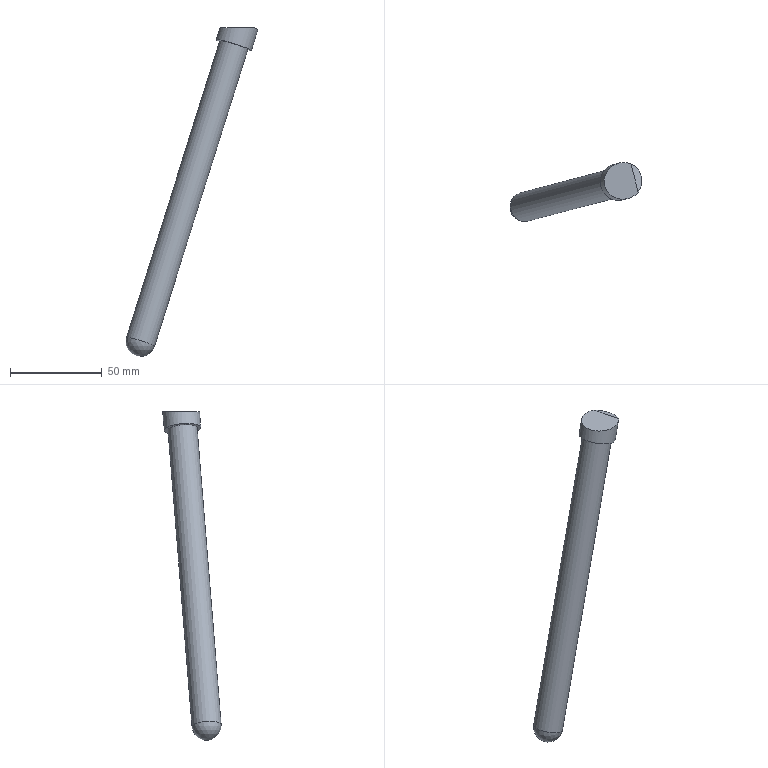Part | STEP file | 车灯-后视镜_id10_x_t | 1 solid | 6 faces | box 72 x 31.93 x 179.239 mm | volume 38387 mm3 | plane 3 | cylinder 2 | sphere 1 | commonest cylinder face diameters 16 x1 20 x1
STEP:
#1=CARTESIAN_POINT('',(-131.667,-129.696,-20.839));
#2=VERTEX_POINT('',#1);
#3=CARTESIAN_POINT('',(-124.036,-129.696,-23.239));
#4=DIRECTION('',(0.2992,0.07718,0.9511));
#5=DIRECTION('',(-0.9539,0.,0.3001));
#6=AXIS2_PLACEMENT_3D('',#3,#4,#5);
#7=CIRCLE('',#6,8.);
#8=EDGE_CURVE('',#2,#2,#7,.T.);
#9=ORIENTED_EDGE('',*,*,#8,.T.);
#10=EDGE_LOOP('',(#9));
#11=FACE_BOUND('',#10,.T.);
#12=CARTESIAN_POINT('',(-65.537,-116.575,136.039));
#13=VERTEX_POINT('',#12);
#14=CARTESIAN_POINT('',(-73.168,-116.575,138.44));
#15=DIRECTION('',(-0.2992,-0.07718,-0.9511));
#16=DIRECTION('',(0.9539,0.,-0.3001));
#17=AXIS2_PLACEMENT_3D('',#14,#15,#16);
#18=CIRCLE('',#17,8.);
#19=EDGE_CURVE('',#13,#13,#18,.T.);
#20=ORIENTED_EDGE('',*,*,#19,.T.);
#21=EDGE_LOOP('',(#20));
#22=FACE_BOUND('',#21,.T.);
#23=CARTESIAN_POINT('',(-92.019,-121.437,78.524));
#24=DIRECTION('',(-0.2992,-0.07718,-0.9511));
#25=DIRECTION('',(-0.9541,0.01184,0.2992));
#26=AXIS2_PLACEMENT_3D('',#23,#24,#25);
#27=CYLINDRICAL_SURFACE('',#26,8.);
#28=ADVANCED_FACE('',(#11,#22),#27,.T.);
#29=ORIENTED_EDGE('',*,*,#8,.F.);
#30=EDGE_LOOP('',(#29));
#31=FACE_OUTER_BOUND('',#30,.T.);
#32=CARTESIAN_POINT('',(-124.036,-129.696,-23.239));
#33=DIRECTION('',(0.,0.,1.));
#34=DIRECTION('',(1.,0.,0.));
#35=AXIS2_PLACEMENT_3D('',#32,#33,#34);
#36=SPHERICAL_SURFACE('',#35,8.);
#37=ADVANCED_FACE('',(#31),#36,.T.);
#38=CARTESIAN_POINT('',(-82.707,-116.575,141.441));
#39=VERTEX_POINT('',#38);
#40=CARTESIAN_POINT('',(-73.168,-116.575,138.44));
#41=DIRECTION('',(-0.2992,-0.07718,-0.9511));
#42=DIRECTION('',(-0.9539,0.,0.3001));
#43=AXIS2_PLACEMENT_3D('',#40,#41,#42);
#44=CIRCLE('',#43,10.);
#45=EDGE_CURVE('',#39,#39,#44,.T.);
#46=ORIENTED_EDGE('',*,*,#45,.T.);
#47=EDGE_LOOP('',(#46));
#48=FACE_BOUND('',#47,.T.);
#49=ORIENTED_EDGE('',*,*,#19,.F.);
#50=EDGE_LOOP('',(#49));
#51=FACE_BOUND('',#50,.T.);
#52=CARTESIAN_POINT('',(-73.168,-116.575,138.44));
#53=DIRECTION('',(0.2992,0.07718,0.9511));
#54=DIRECTION('',(0.9539,0.,-0.3001));
#55=AXIS2_PLACEMENT_3D('',#52,#53,#54);
#56=PLANE('',#55);
#57=ADVANCED_FACE('',(#48,#51),#56,.F.);
#58=CARTESIAN_POINT('',(-66.054,-106.475,148.));
#59=VERTEX_POINT('',#58);
#60=CARTESIAN_POINT('',(-62.057,-121.974,148.));
#61=VERTEX_POINT('',#60);
#62=CARTESIAN_POINT('',(-70.16,-115.799,148.));
#63=DIRECTION('',(0.,0.,1.));
#64=DIRECTION('',(-0.9683,-0.2498,0.));
#65=AXIS2_PLACEMENT_3D('',#62,#63,#64);
#66=ELLIPSE('',#65,10.515,10.);
#67=EDGE_CURVE('',#59,#61,#66,.T.);
#68=ORIENTED_EDGE('',*,*,#67,.F.);
#69=CARTESIAN_POINT('',(-69.577,-115.649,149.853));
#70=DIRECTION('',(-0.2992,-0.07718,-0.9511));
#71=DIRECTION('',(-0.9539,0.,0.3001));
#72=AXIS2_PLACEMENT_3D('',#69,#70,#71);
#73=CIRCLE('',#72,10.);
#74=EDGE_CURVE('',#59,#61,#73,.T.);
#75=ORIENTED_EDGE('',*,*,#74,.T.);
#76=EDGE_LOOP('',(#68,#75));
#77=FACE_BOUND('',#76,.T.);
#78=ORIENTED_EDGE('',*,*,#45,.F.);
#79=EDGE_LOOP('',(#78));
#80=FACE_BOUND('',#79,.T.);
#81=CARTESIAN_POINT('',(-69.577,-115.649,149.853));
#82=DIRECTION('',(-0.2992,-0.07718,-0.9511));
#83=DIRECTION('',(-0.9539,0.,0.3001));
#84=AXIS2_PLACEMENT_3D('',#81,#82,#83);
#85=CYLINDRICAL_SURFACE('',#84,10.);
#86=ADVANCED_FACE('',(#77,#80),#85,.T.);
#87=CARTESIAN_POINT('',(-64.056,-114.224,148.));
#88=DIRECTION('',(-0.2498,0.9683,0.));
#89=VECTOR('',#88,1.);
#90=LINE('',#87,#89);
#91=EDGE_CURVE('',#61,#59,#90,.T.);
#92=ORIENTED_EDGE('',*,*,#91,.F.);
#93=ORIENTED_EDGE('',*,*,#74,.F.);
#94=EDGE_LOOP('',(#92,#93));
#95=FACE_OUTER_BOUND('',#94,.T.);
#96=CARTESIAN_POINT('',(-69.577,-115.649,149.853));
#97=DIRECTION('',(0.2992,0.07718,0.9511));
#98=DIRECTION('',(0.9541,-0.01184,-0.2992));
#99=AXIS2_PLACEMENT_3D('',#96,#97,#98);
#100=PLANE('',#99);
#101=ADVANCED_FACE('',(#95),#100,.T.);
#102=ORIENTED_EDGE('',*,*,#67,.T.);
#103=ORIENTED_EDGE('',*,*,#91,.T.);
#104=EDGE_LOOP('',(#102,#103));
#105=FACE_OUTER_BOUND('',#104,.T.);
#106=CARTESIAN_POINT('',(-125.,-190.,148.));
#107=DIRECTION('',(0.,0.,-1.));
#108=DIRECTION('',(-1.,0.,0.));
#109=AXIS2_PLACEMENT_3D('',#106,#107,#108);
#110=PLANE('',#109);
#111=ADVANCED_FACE('',(#105),#110,.F.);
#112=CLOSED_SHELL('',(#28,#37,#57,#86,#101,#111));
#113=MANIFOLD_SOLID_BREP('',#112);
#114=(LENGTH_UNIT()NAMED_UNIT(*)SI_UNIT(.MILLI.,.METRE.));
#115=UNCERTAINTY_MEASURE_WITH_UNIT(LENGTH_MEASURE(0.00002),#114,'','');
#116=(NAMED_UNIT(*)PLANE_ANGLE_UNIT()SI_UNIT($,.RADIAN.));
#117=PLANE_ANGLE_MEASURE_WITH_UNIT(PLANE_ANGLE_MEASURE(0.01745),#116);
#118=DIMENSIONAL_EXPONENTS(0.,0.,0.,0.,0.,0.,0.);
#119=(CONVERSION_BASED_UNIT('DEGREE',#117)NAMED_UNIT(#118)PLANE_ANGLE_UNIT());
#120=(NAMED_UNIT(*)SI_UNIT($,.STERADIAN.)SOLID_ANGLE_UNIT());
#121=(GEOMETRIC_REPRESENTATION_CONTEXT(3)GLOBAL_UNCERTAINTY_ASSIGNED_CONTEXT((#115))GLOBAL_UNIT_ASSIGNED_CONTEXT((#114,#119,#120))REPRESENTATION_CONTEXT('',''));
#122=ADVANCED_BREP_SHAPE_REPRESENTATION('',(#113),#121);